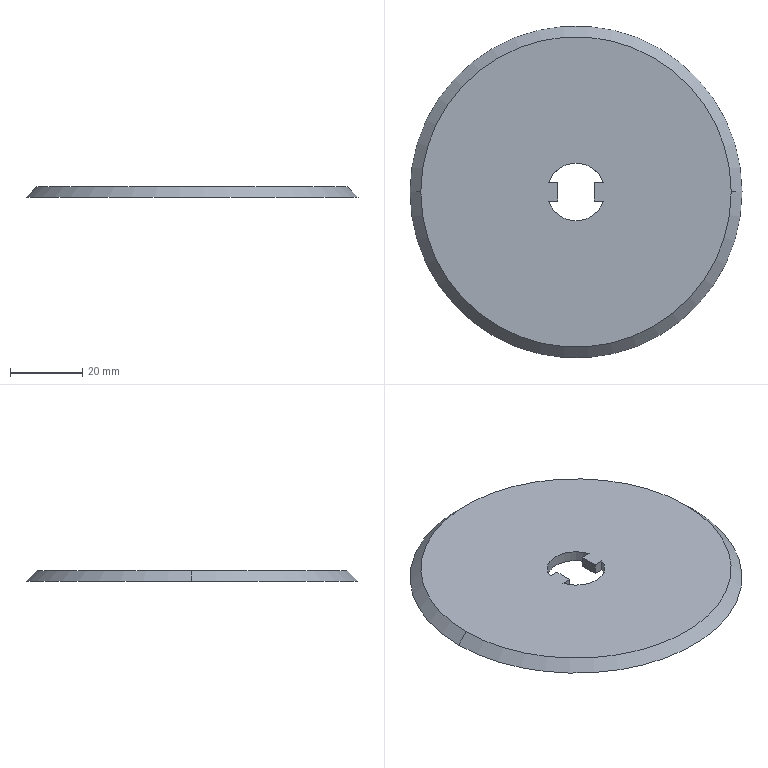Part | SolidWorks | features Chamfer 1, Extrusion 1, ICE 1 | 1 solid | 12 faces | box 92 x 92 x 3 mm | volume 18153 mm3 | plane 8 | cone 2 | cylinder 2 | commonest cylinder face diameters 16 x2
STEP:
#1=CARTESIAN_POINT('',(43.,0.,3.));
#2=VERTEX_POINT('',#1);
#3=CARTESIAN_POINT('',(-43.,0.,3.));
#4=VERTEX_POINT('',#3);
#5=CARTESIAN_POINT('',(0.,0.,3.));
#6=DIRECTION('',(0.,0.,1.));
#7=DIRECTION('',(1.,0.,0.));
#8=AXIS2_PLACEMENT_3D('',#5,#6,#7);
#9=CIRCLE('',#8,43.);
#10=EDGE_CURVE('',#2,#4,#9,.T.);
#11=ORIENTED_EDGE('',*,*,#10,.F.);
#12=CARTESIAN_POINT('',(46.,0.,0.));
#13=VERTEX_POINT('',#12);
#14=CARTESIAN_POINT('',(43.,0.,3.));
#15=DIRECTION('',(0.7071,0.,-0.7071));
#16=VECTOR('',#15,1000.);
#17=LINE('',#14,#16);
#18=EDGE_CURVE('',#2,#13,#17,.T.);
#19=ORIENTED_EDGE('',*,*,#18,.T.);
#20=CARTESIAN_POINT('',(-46.,0.,0.));
#21=VERTEX_POINT('',#20);
#22=CARTESIAN_POINT('',(0.,0.,0.));
#23=DIRECTION('',(0.,0.,1.));
#24=DIRECTION('',(1.,0.,0.));
#25=AXIS2_PLACEMENT_3D('',#22,#23,#24);
#26=CIRCLE('',#25,46.);
#27=EDGE_CURVE('',#13,#21,#26,.T.);
#28=ORIENTED_EDGE('',*,*,#27,.T.);
#29=CARTESIAN_POINT('',(-43.,0.,3.));
#30=DIRECTION('',(-0.7071,0.,-0.7071));
#31=VECTOR('',#30,1000.);
#32=LINE('',#29,#31);
#33=EDGE_CURVE('',#4,#21,#32,.T.);
#34=ORIENTED_EDGE('',*,*,#33,.F.);
#35=EDGE_LOOP('',(#11,#19,#28,#34));
#36=FACE_OUTER_BOUND('',#35,.T.);
#37=CARTESIAN_POINT('',(0.,0.,3.));
#38=DIRECTION('',(0.,0.,-1.));
#39=DIRECTION('',(-1.,0.,0.));
#40=AXIS2_PLACEMENT_3D('',#37,#38,#39);
#41=CONICAL_SURFACE('',#40,43.,0.7854);
#42=ADVANCED_FACE('',(#36),#41,.T.);
#43=CARTESIAN_POINT('',(7.599,2.5,3.));
#44=VERTEX_POINT('',#43);
#45=CARTESIAN_POINT('',(7.599,2.5,0.));
#46=VERTEX_POINT('',#45);
#47=CARTESIAN_POINT('',(7.599,2.5,3.));
#48=DIRECTION('',(0.,0.,-1.));
#49=VECTOR('',#48,1000.);
#50=LINE('',#47,#49);
#51=EDGE_CURVE('',#44,#46,#50,.T.);
#52=ORIENTED_EDGE('',*,*,#51,.F.);
#53=CARTESIAN_POINT('',(-7.599,2.5,3.));
#54=VERTEX_POINT('',#53);
#55=CARTESIAN_POINT('',(0.,0.,3.));
#56=DIRECTION('',(0.,0.,1.));
#57=DIRECTION('',(1.,0.,0.));
#58=AXIS2_PLACEMENT_3D('',#55,#56,#57);
#59=CIRCLE('',#58,8.);
#60=EDGE_CURVE('',#44,#54,#59,.T.);
#61=ORIENTED_EDGE('',*,*,#60,.T.);
#62=CARTESIAN_POINT('',(-7.599,2.5,0.));
#63=VERTEX_POINT('',#62);
#64=CARTESIAN_POINT('',(-7.599,2.5,3.));
#65=DIRECTION('',(0.,0.,1.));
#66=VECTOR('',#65,1000.);
#67=LINE('',#64,#66);
#68=EDGE_CURVE('',#63,#54,#67,.T.);
#69=ORIENTED_EDGE('',*,*,#68,.F.);
#70=CARTESIAN_POINT('',(0.,0.,0.));
#71=DIRECTION('',(0.,0.,1.));
#72=DIRECTION('',(1.,0.,0.));
#73=AXIS2_PLACEMENT_3D('',#70,#71,#72);
#74=CIRCLE('',#73,8.);
#75=EDGE_CURVE('',#46,#63,#74,.T.);
#76=ORIENTED_EDGE('',*,*,#75,.F.);
#77=EDGE_LOOP('',(#52,#61,#69,#76));
#78=FACE_OUTER_BOUND('',#77,.T.);
#79=CARTESIAN_POINT('',(0.,0.,3.));
#80=DIRECTION('',(0.,0.,-1.));
#81=DIRECTION('',(-1.,0.,0.));
#82=AXIS2_PLACEMENT_3D('',#79,#80,#81);
#83=CYLINDRICAL_SURFACE('',#82,8.);
#84=ADVANCED_FACE('',(#78),#83,.F.);
#85=CARTESIAN_POINT('',(0.,0.,3.));
#86=DIRECTION('',(0.,0.,1.));
#87=DIRECTION('',(1.,0.,0.));
#88=AXIS2_PLACEMENT_3D('',#85,#86,#87);
#89=CIRCLE('',#88,43.);
#90=EDGE_CURVE('',#4,#2,#89,.T.);
#91=ORIENTED_EDGE('',*,*,#90,.T.);
#92=ORIENTED_EDGE('',*,*,#10,.T.);
#93=EDGE_LOOP('',(#91,#92));
#94=FACE_OUTER_BOUND('',#93,.T.);
#95=ORIENTED_EDGE('',*,*,#60,.F.);
#96=CARTESIAN_POINT('',(5.,2.5,3.));
#97=VERTEX_POINT('',#96);
#98=CARTESIAN_POINT('',(5.,2.5,3.));
#99=DIRECTION('',(-1.,0.,0.));
#100=VECTOR('',#99,1000.);
#101=LINE('',#98,#100);
#102=EDGE_CURVE('',#44,#97,#101,.T.);
#103=ORIENTED_EDGE('',*,*,#102,.T.);
#104=CARTESIAN_POINT('',(5.,-2.5,3.));
#105=VERTEX_POINT('',#104);
#106=CARTESIAN_POINT('',(5.,2.5,3.));
#107=DIRECTION('',(0.,-1.,0.));
#108=VECTOR('',#107,1000.);
#109=LINE('',#106,#108);
#110=EDGE_CURVE('',#97,#105,#109,.T.);
#111=ORIENTED_EDGE('',*,*,#110,.T.);
#112=CARTESIAN_POINT('',(7.599,-2.5,3.));
#113=VERTEX_POINT('',#112);
#114=CARTESIAN_POINT('',(5.,-2.5,3.));
#115=DIRECTION('',(1.,0.,0.));
#116=VECTOR('',#115,1000.);
#117=LINE('',#114,#116);
#118=EDGE_CURVE('',#105,#113,#117,.T.);
#119=ORIENTED_EDGE('',*,*,#118,.T.);
#120=CARTESIAN_POINT('',(-7.599,-2.5,3.));
#121=VERTEX_POINT('',#120);
#122=CARTESIAN_POINT('',(0.,0.,3.));
#123=DIRECTION('',(0.,0.,1.));
#124=DIRECTION('',(1.,0.,0.));
#125=AXIS2_PLACEMENT_3D('',#122,#123,#124);
#126=CIRCLE('',#125,8.);
#127=EDGE_CURVE('',#121,#113,#126,.T.);
#128=ORIENTED_EDGE('',*,*,#127,.F.);
#129=CARTESIAN_POINT('',(-5.,-2.5,3.));
#130=VERTEX_POINT('',#129);
#131=CARTESIAN_POINT('',(-15.,-2.5,3.));
#132=DIRECTION('',(1.,0.,0.));
#133=VECTOR('',#132,1000.);
#134=LINE('',#131,#133);
#135=EDGE_CURVE('',#121,#130,#134,.T.);
#136=ORIENTED_EDGE('',*,*,#135,.T.);
#137=CARTESIAN_POINT('',(-5.,2.5,3.));
#138=VERTEX_POINT('',#137);
#139=CARTESIAN_POINT('',(-5.,2.5,3.));
#140=DIRECTION('',(0.,1.,0.));
#141=VECTOR('',#140,1000.);
#142=LINE('',#139,#141);
#143=EDGE_CURVE('',#130,#138,#142,.T.);
#144=ORIENTED_EDGE('',*,*,#143,.T.);
#145=CARTESIAN_POINT('',(-15.,2.5,3.));
#146=DIRECTION('',(-1.,0.,0.));
#147=VECTOR('',#146,1000.);
#148=LINE('',#145,#147);
#149=EDGE_CURVE('',#138,#54,#148,.T.);
#150=ORIENTED_EDGE('',*,*,#149,.T.);
#151=EDGE_LOOP('',(#95,#103,#111,#119,#128,#136,#144,#150));
#152=FACE_BOUND('',#151,.T.);
#153=CARTESIAN_POINT('',(0.,0.,3.));
#154=DIRECTION('',(0.,0.,1.));
#155=DIRECTION('',(1.,0.,0.));
#156=AXIS2_PLACEMENT_3D('',#153,#154,#155);
#157=PLANE('',#156);
#158=ADVANCED_FACE('',(#94,#152),#157,.T.);
#159=CARTESIAN_POINT('',(5.,2.5,0.));
#160=VERTEX_POINT('',#159);
#161=CARTESIAN_POINT('',(5.,2.5,0.));
#162=DIRECTION('',(-1.,0.,0.));
#163=VECTOR('',#162,1000.);
#164=LINE('',#161,#163);
#165=EDGE_CURVE('',#46,#160,#164,.T.);
#166=ORIENTED_EDGE('',*,*,#165,.F.);
#167=ORIENTED_EDGE('',*,*,#75,.T.);
#168=CARTESIAN_POINT('',(-5.,2.5,0.));
#169=VERTEX_POINT('',#168);
#170=CARTESIAN_POINT('',(-15.,2.5,0.));
#171=DIRECTION('',(-1.,0.,0.));
#172=VECTOR('',#171,1000.);
#173=LINE('',#170,#172);
#174=EDGE_CURVE('',#169,#63,#173,.T.);
#175=ORIENTED_EDGE('',*,*,#174,.F.);
#176=CARTESIAN_POINT('',(-5.,-2.5,0.));
#177=VERTEX_POINT('',#176);
#178=CARTESIAN_POINT('',(-5.,2.5,0.));
#179=DIRECTION('',(0.,1.,0.));
#180=VECTOR('',#179,1000.);
#181=LINE('',#178,#180);
#182=EDGE_CURVE('',#177,#169,#181,.T.);
#183=ORIENTED_EDGE('',*,*,#182,.F.);
#184=CARTESIAN_POINT('',(-7.599,-2.5,0.));
#185=VERTEX_POINT('',#184);
#186=CARTESIAN_POINT('',(-15.,-2.5,0.));
#187=DIRECTION('',(1.,0.,0.));
#188=VECTOR('',#187,1000.);
#189=LINE('',#186,#188);
#190=EDGE_CURVE('',#185,#177,#189,.T.);
#191=ORIENTED_EDGE('',*,*,#190,.F.);
#192=CARTESIAN_POINT('',(7.599,-2.5,0.));
#193=VERTEX_POINT('',#192);
#194=CARTESIAN_POINT('',(0.,0.,0.));
#195=DIRECTION('',(0.,0.,1.));
#196=DIRECTION('',(1.,0.,0.));
#197=AXIS2_PLACEMENT_3D('',#194,#195,#196);
#198=CIRCLE('',#197,8.);
#199=EDGE_CURVE('',#185,#193,#198,.T.);
#200=ORIENTED_EDGE('',*,*,#199,.T.);
#201=CARTESIAN_POINT('',(5.,-2.5,0.));
#202=VERTEX_POINT('',#201);
#203=CARTESIAN_POINT('',(5.,-2.5,0.));
#204=DIRECTION('',(1.,0.,0.));
#205=VECTOR('',#204,1000.);
#206=LINE('',#203,#205);
#207=EDGE_CURVE('',#202,#193,#206,.T.);
#208=ORIENTED_EDGE('',*,*,#207,.F.);
#209=CARTESIAN_POINT('',(5.,2.5,0.));
#210=DIRECTION('',(0.,-1.,0.));
#211=VECTOR('',#210,1000.);
#212=LINE('',#209,#211);
#213=EDGE_CURVE('',#160,#202,#212,.T.);
#214=ORIENTED_EDGE('',*,*,#213,.F.);
#215=EDGE_LOOP('',(#166,#167,#175,#183,#191,#200,#208,#214));
#216=FACE_BOUND('',#215,.T.);
#217=CARTESIAN_POINT('',(0.,0.,0.));
#218=DIRECTION('',(0.,0.,1.));
#219=DIRECTION('',(1.,0.,0.));
#220=AXIS2_PLACEMENT_3D('',#217,#218,#219);
#221=CIRCLE('',#220,46.);
#222=EDGE_CURVE('',#21,#13,#221,.T.);
#223=ORIENTED_EDGE('',*,*,#222,.F.);
#224=ORIENTED_EDGE('',*,*,#27,.F.);
#225=EDGE_LOOP('',(#223,#224));
#226=FACE_OUTER_BOUND('',#225,.T.);
#227=CARTESIAN_POINT('',(0.,0.,0.));
#228=DIRECTION('',(0.,0.,1.));
#229=DIRECTION('',(1.,0.,0.));
#230=AXIS2_PLACEMENT_3D('',#227,#228,#229);
#231=PLANE('',#230);
#232=ADVANCED_FACE('',(#216,#226),#231,.F.);
#233=CARTESIAN_POINT('',(7.599,-2.5,3.));
#234=DIRECTION('',(0.,0.,1.));
#235=VECTOR('',#234,1000.);
#236=LINE('',#233,#235);
#237=EDGE_CURVE('',#193,#113,#236,.T.);
#238=ORIENTED_EDGE('',*,*,#237,.F.);
#239=ORIENTED_EDGE('',*,*,#199,.F.);
#240=CARTESIAN_POINT('',(-7.599,-2.5,3.));
#241=DIRECTION('',(0.,0.,-1.));
#242=VECTOR('',#241,1000.);
#243=LINE('',#240,#242);
#244=EDGE_CURVE('',#121,#185,#243,.T.);
#245=ORIENTED_EDGE('',*,*,#244,.F.);
#246=ORIENTED_EDGE('',*,*,#127,.T.);
#247=EDGE_LOOP('',(#238,#239,#245,#246));
#248=FACE_OUTER_BOUND('',#247,.T.);
#249=CARTESIAN_POINT('',(0.,0.,3.));
#250=DIRECTION('',(0.,0.,-1.));
#251=DIRECTION('',(-1.,0.,0.));
#252=AXIS2_PLACEMENT_3D('',#249,#250,#251);
#253=CYLINDRICAL_SURFACE('',#252,8.);
#254=ADVANCED_FACE('',(#248),#253,.F.);
#255=ORIENTED_EDGE('',*,*,#174,.T.);
#256=ORIENTED_EDGE('',*,*,#68,.T.);
#257=ORIENTED_EDGE('',*,*,#149,.F.);
#258=CARTESIAN_POINT('',(-5.,2.5,0.));
#259=DIRECTION('',(0.,0.,1.));
#260=VECTOR('',#259,1000.);
#261=LINE('',#258,#260);
#262=EDGE_CURVE('',#169,#138,#261,.T.);
#263=ORIENTED_EDGE('',*,*,#262,.F.);
#264=EDGE_LOOP('',(#255,#256,#257,#263));
#265=FACE_OUTER_BOUND('',#264,.T.);
#266=CARTESIAN_POINT('',(-15.,2.5,0.));
#267=DIRECTION('',(0.,1.,0.));
#268=DIRECTION('',(-1.,0.,0.));
#269=AXIS2_PLACEMENT_3D('',#266,#267,#268);
#270=PLANE('',#269);
#271=ADVANCED_FACE('',(#265),#270,.T.);
#272=ORIENTED_EDGE('',*,*,#143,.F.);
#273=CARTESIAN_POINT('',(-5.,-2.5,0.));
#274=DIRECTION('',(0.,0.,1.));
#275=VECTOR('',#274,1000.);
#276=LINE('',#273,#275);
#277=EDGE_CURVE('',#177,#130,#276,.T.);
#278=ORIENTED_EDGE('',*,*,#277,.F.);
#279=ORIENTED_EDGE('',*,*,#182,.T.);
#280=ORIENTED_EDGE('',*,*,#262,.T.);
#281=EDGE_LOOP('',(#272,#278,#279,#280));
#282=FACE_OUTER_BOUND('',#281,.T.);
#283=CARTESIAN_POINT('',(-5.,2.5,0.));
#284=DIRECTION('',(1.,0.,0.));
#285=DIRECTION('',(0.,0.,-1.));
#286=AXIS2_PLACEMENT_3D('',#283,#284,#285);
#287=PLANE('',#286);
#288=ADVANCED_FACE('',(#282),#287,.T.);
#289=ORIENTED_EDGE('',*,*,#135,.F.);
#290=ORIENTED_EDGE('',*,*,#244,.T.);
#291=ORIENTED_EDGE('',*,*,#190,.T.);
#292=ORIENTED_EDGE('',*,*,#277,.T.);
#293=EDGE_LOOP('',(#289,#290,#291,#292));
#294=FACE_OUTER_BOUND('',#293,.T.);
#295=CARTESIAN_POINT('',(-15.,-2.5,0.));
#296=DIRECTION('',(0.,-1.,0.));
#297=DIRECTION('',(1.,0.,0.));
#298=AXIS2_PLACEMENT_3D('',#295,#296,#297);
#299=PLANE('',#298);
#300=ADVANCED_FACE('',(#294),#299,.T.);
#301=ORIENTED_EDGE('',*,*,#110,.F.);
#302=CARTESIAN_POINT('',(5.,2.5,0.));
#303=DIRECTION('',(0.,0.,1.));
#304=VECTOR('',#303,1000.);
#305=LINE('',#302,#304);
#306=EDGE_CURVE('',#160,#97,#305,.T.);
#307=ORIENTED_EDGE('',*,*,#306,.F.);
#308=ORIENTED_EDGE('',*,*,#213,.T.);
#309=CARTESIAN_POINT('',(5.,-2.5,0.));
#310=DIRECTION('',(0.,0.,1.));
#311=VECTOR('',#310,1000.);
#312=LINE('',#309,#311);
#313=EDGE_CURVE('',#202,#105,#312,.T.);
#314=ORIENTED_EDGE('',*,*,#313,.T.);
#315=EDGE_LOOP('',(#301,#307,#308,#314));
#316=FACE_OUTER_BOUND('',#315,.T.);
#317=CARTESIAN_POINT('',(5.,2.5,0.));
#318=DIRECTION('',(-1.,0.,0.));
#319=DIRECTION('',(0.,0.,1.));
#320=AXIS2_PLACEMENT_3D('',#317,#318,#319);
#321=PLANE('',#320);
#322=ADVANCED_FACE('',(#316),#321,.T.);
#323=ORIENTED_EDGE('',*,*,#102,.F.);
#324=ORIENTED_EDGE('',*,*,#51,.T.);
#325=ORIENTED_EDGE('',*,*,#165,.T.);
#326=ORIENTED_EDGE('',*,*,#306,.T.);
#327=EDGE_LOOP('',(#323,#324,#325,#326));
#328=FACE_OUTER_BOUND('',#327,.T.);
#329=CARTESIAN_POINT('',(5.,2.5,0.));
#330=DIRECTION('',(0.,1.,0.));
#331=DIRECTION('',(-1.,0.,0.));
#332=AXIS2_PLACEMENT_3D('',#329,#330,#331);
#333=PLANE('',#332);
#334=ADVANCED_FACE('',(#328),#333,.T.);
#335=ORIENTED_EDGE('',*,*,#207,.T.);
#336=ORIENTED_EDGE('',*,*,#237,.T.);
#337=ORIENTED_EDGE('',*,*,#118,.F.);
#338=ORIENTED_EDGE('',*,*,#313,.F.);
#339=EDGE_LOOP('',(#335,#336,#337,#338));
#340=FACE_OUTER_BOUND('',#339,.T.);
#341=CARTESIAN_POINT('',(5.,-2.5,0.));
#342=DIRECTION('',(0.,-1.,0.));
#343=DIRECTION('',(1.,0.,0.));
#344=AXIS2_PLACEMENT_3D('',#341,#342,#343);
#345=PLANE('',#344);
#346=ADVANCED_FACE('',(#340),#345,.T.);
#347=ORIENTED_EDGE('',*,*,#18,.F.);
#348=ORIENTED_EDGE('',*,*,#90,.F.);
#349=ORIENTED_EDGE('',*,*,#33,.T.);
#350=ORIENTED_EDGE('',*,*,#222,.T.);
#351=EDGE_LOOP('',(#347,#348,#349,#350));
#352=FACE_OUTER_BOUND('',#351,.T.);
#353=CARTESIAN_POINT('',(0.,0.,3.));
#354=DIRECTION('',(0.,0.,-1.));
#355=DIRECTION('',(-1.,0.,0.));
#356=AXIS2_PLACEMENT_3D('',#353,#354,#355);
#357=CONICAL_SURFACE('',#356,43.,0.7854);
#358=ADVANCED_FACE('',(#352),#357,.T.);
#359=CLOSED_SHELL('',(#42,#84,#158,#232,#254,#271,#288,#300,#322,#334,#346,#358));
#360=MANIFOLD_SOLID_BREP('',#359);
#361=CARTESIAN_POINT('',(0.,0.,0.));
#362=DIRECTION('',(0.,0.,1.));
#363=DIRECTION('',(1.,0.,0.));
#364=AXIS2_PLACEMENT_3D('',#361,#362,#363);
#365=(LENGTH_UNIT()NAMED_UNIT(*)SI_UNIT(.MILLI.,.METRE.));
#366=UNCERTAINTY_MEASURE_WITH_UNIT(LENGTH_MEASURE(0.00001),#365,'','');
#367=(NAMED_UNIT(*)PLANE_ANGLE_UNIT()SI_UNIT($,.RADIAN.));
#368=(NAMED_UNIT(*)SI_UNIT($,.STERADIAN.)SOLID_ANGLE_UNIT());
#369=(GEOMETRIC_REPRESENTATION_CONTEXT(3)GLOBAL_UNCERTAINTY_ASSIGNED_CONTEXT((#366))GLOBAL_UNIT_ASSIGNED_CONTEXT((#365,#367,#368))REPRESENTATION_CONTEXT('',''));
#370=ADVANCED_BREP_SHAPE_REPRESENTATION('',(#360,#364),#369);